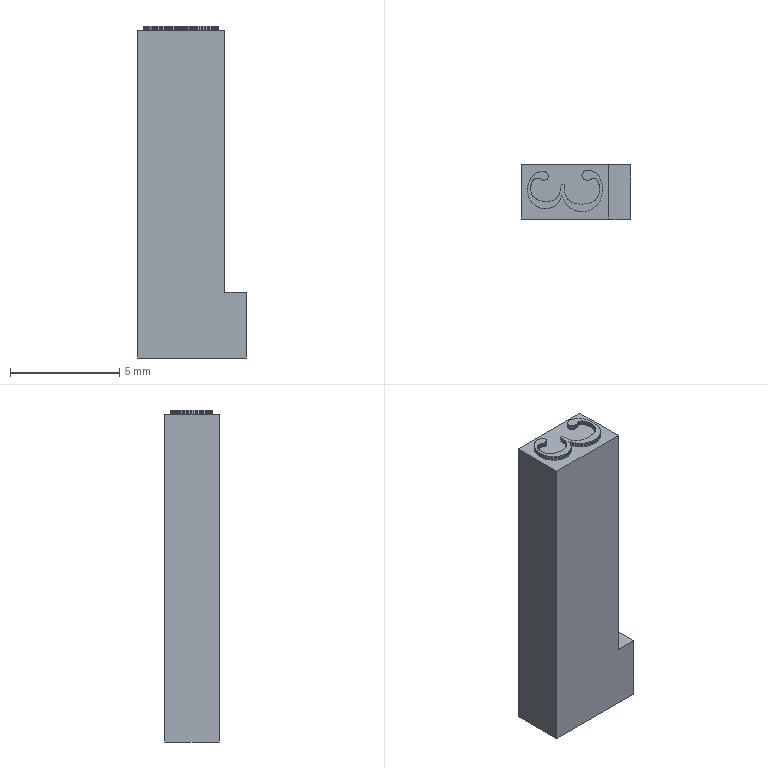Part | NX | features DIE-32 2 | 1 solid | 307 faces | box 5 x 2.5 x 15.2 mm | volume 157.861 mm3 | plane 307